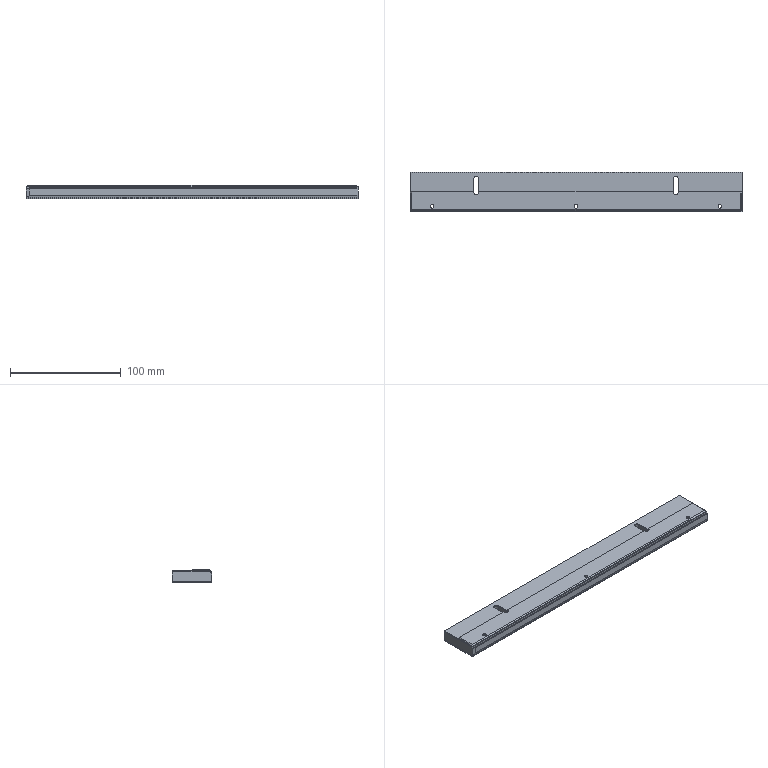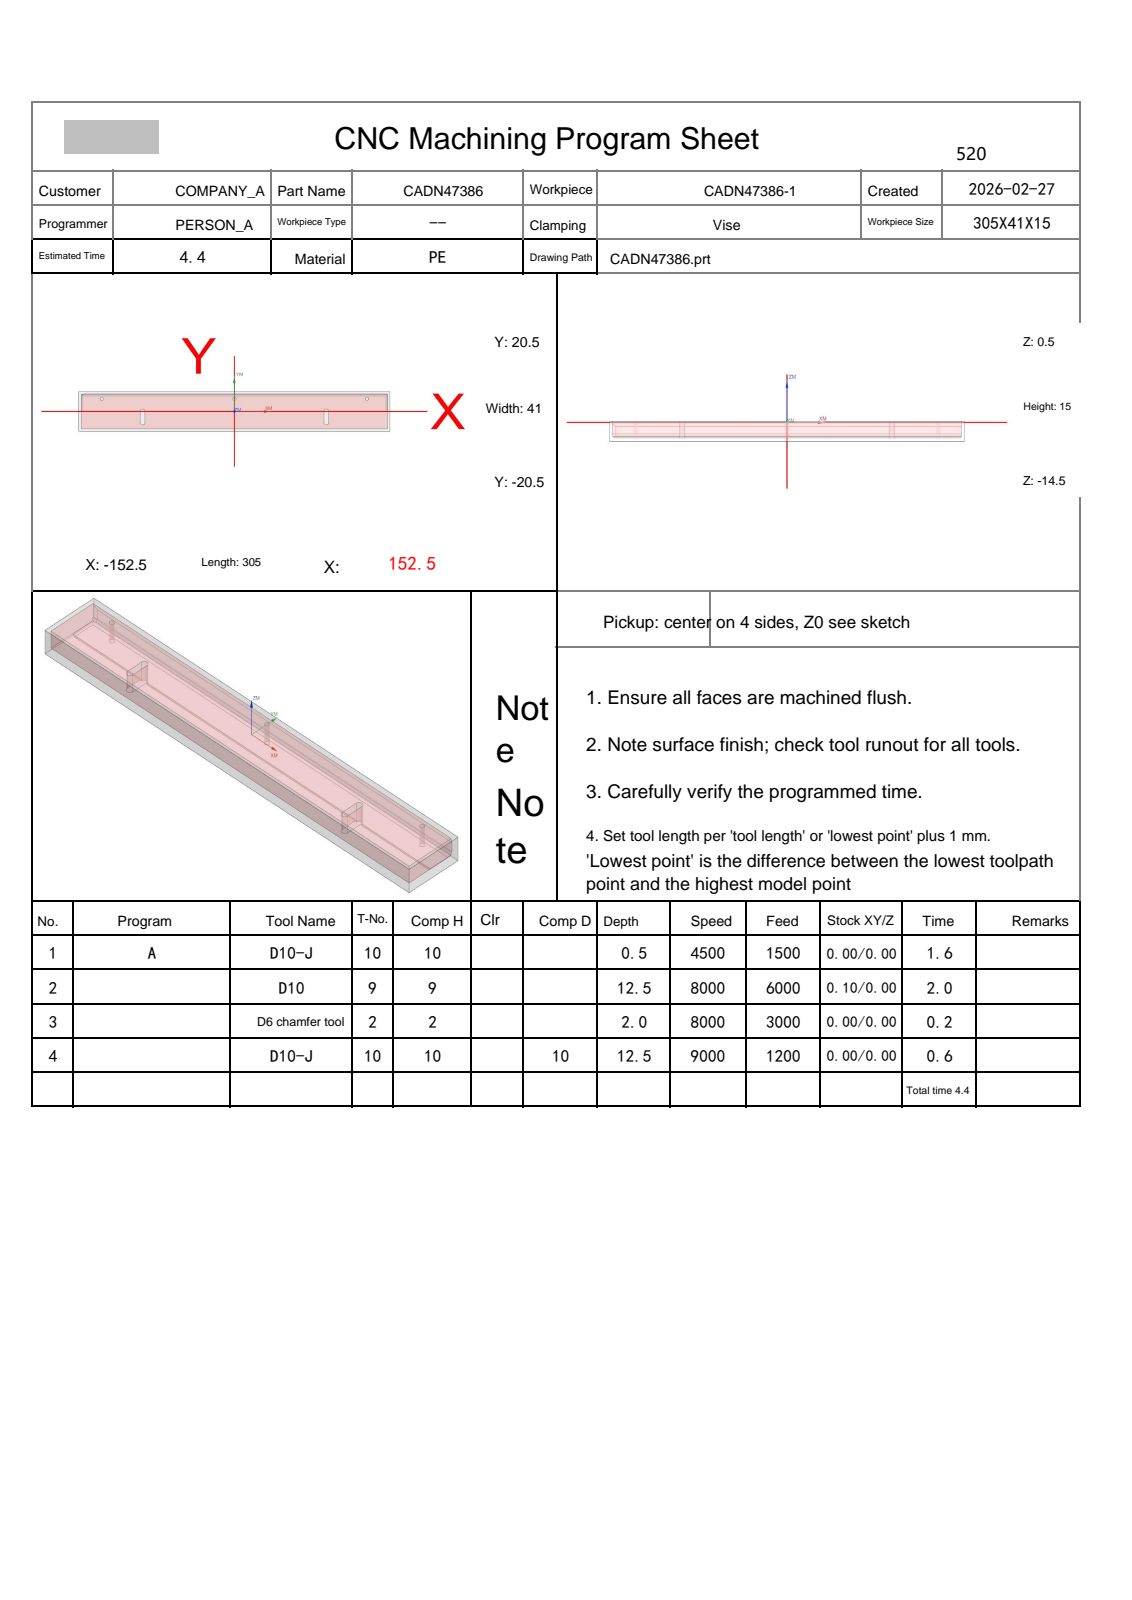NC program | NX | posted by the shop | part box 300 x 36 x 12 mm
Whole program:
%
O0001
(Machine time: 5.25 MIN)
(===Total Tool:3===)
(T10=D10-J  D=10.  R=0.   D-  H10 Z=-12.  )
(T9=D10     D=10.  R=0.   D-  H09 Z=-12.  )
(T2=D6 chamfer tool   D=6.   R=0.   D-  H02 Z=-1.5  )
G80 G90 G17 G49 G40
G91 G28 Z0
M01
N1 T10 M06
(D10-J  D=10. R=0. H=10 ce=0.00 di=0.00)
G00 G90 G54 X140.111 Y28. M03 S4500
G43 H10 Z29.
M08
Z2.
G01 Z0.0 F1500.
X145.111 Y23.
X155. Y13.111
Y3.222
X135.222 Y23.
X125.333
X155. Y-6.667
Y-16.556
X115.444 Y23.
X105.556
X151.556 Y-23.
X141.667
X95.667 Y23.
X85.778
X131.778 Y-23.
X121.889
X75.889 Y23.
X66.
X112. Y-23.
X102.111
X56.111 Y23.
X46.222
X92.222 Y-23.
X82.333
X36.333 Y23.
X26.444
X72.444 Y-23.
X62.556
X16.556 Y23.
X6.667
X52.667 Y-23.
X42.778
X-3.222 Y23.
X-13.111
X32.889 Y-23.
X23.
X-23. Y23.
X-32.889
X13.111 Y-23.
X3.222
X-42.778 Y23.
X-52.667
X-6.667 Y-23.
X-16.556
X-62.556 Y23.
X-72.444
X-26.444 Y-23.
X-36.333
X-82.333 Y23.
X-92.222
X-46.222 Y-23.
X-56.111
X-102.111 Y23.
X-112.
X-66. Y-23.
X-75.889
X-121.889 Y23.
X-131.778
X-85.778 Y-23.
X-95.667
X-141.667 Y23.
X-151.556
X-105.556 Y-23.
X-115.444
X-155. Y16.556
Y6.667
X-125.333 Y-23.
X-135.222
X-155. Y-3.222
Y-13.111
X-145.111 Y-23.
X-140.111 Y-28.
Z2.
G00 Z29.
G91 G28 Z0.0
M05
M09
G91 G28 Z0.0
M01
N2 T09 M06
(D10  D=10. R=0. H=09 ce=0.10 di=0.00)
G00 G90 G54 X-.443 Y23.1 M03 S8000
G43 H09 Z29.
M08
Z.5
G01 X150. Z.333 F6000.
G02 X155.1 Y18. Z.324 I0.0 J-5.1
G01 Y-18. Z.284
G02 X150. Y-23.1 Z.275 I-5.1 J0.0
G01 X-150. Z-.058
G02 X-155.1 Y-18. Z-.067 I0.0 J5.1
G01 Y17.5 Z-.106
G02 X-150.838 Y22.531 Z-.114 I5.1 J0.0
G01 X-147.422 Y23.1 Z-.118
X150. Z-.448
G02 X155.1 Y18. Z-.457 I0.0 J-5.1
G01 Y-18. Z-.497
G02 X150. Y-23.1 Z-.506 I-5.1 J0.0
G01 X-150. Z-.839
G02 X-155.1 Y-18. Z-.848 I0.0 J5.1
G01 Y17.5 Z-.887
G02 X-150.838 Y22.531 Z-.895 I5.1 J0.0
G01 X-147.422 Y23.1 Z-.899
X150. Z-1.23
G02 X155.1 Y18. Z-1.238 I0.0 J-5.1
G01 Y-18. Z-1.278
G02 X150. Y-23.1 Z-1.287 I-5.1 J0.0
G01 X-150. Z-1.62
G02 X-155.1 Y-18. Z-1.629 I0.0 J5.1
G01 Y17.5 Z-1.669
G02 X-150.838 Y22.531 Z-1.677 I5.1 J0.0
G01 X-147.422 Y23.1 Z-1.681
X150. Z-2.011
G02 X155.1 Y18. Z-2.02 I0.0 J-5.1
G01 Y-18. Z-2.06
G02 X150. Y-23.1 Z-2.069 I-5.1 J0.0
G01 X-150. Z-2.402
G02 X-155.1 Y-18. Z-2.411 I0.0 J5.1
G01 Y17.5 Z-2.45
G02 X-150.838 Y22.531 Z-2.458 I5.1 J0.0
G01 X-147.422 Y23.1 Z-2.462
X150. Z-2.792
G02 X155.1 Y18. Z-2.801 I0.0 J-5.1
G01 Y-18. Z-2.841
G02 X150. Y-23.1 Z-2.85 I-5.1 J0.0
G01 X-150. Z-3.183
G02 X-155.1 Y-18. Z-3.192 I0.0 J5.1
G01 Y17.5 Z-3.231
G02 X-150.838 Y22.531 Z-3.239 I5.1 J0.0
G01 X-147.422 Y23.1 Z-3.243
X150. Z-3.573
G02 X155.1 Y18. Z-3.582 I0.0 J-5.1
G01 Y-18. Z-3.622
G02 X150. Y-23.1 Z-3.631 I-5.1 J0.0
G01 X-150. Z-3.964
G02 X-155.1 Y-18. Z-3.973 I0.0 J5.1
G01 Y17.5 Z-4.012
G02 X-150.838 Y22.531 Z-4.02 I5.1 J0.0
G01 X-147.422 Y23.1 Z-4.024
X150. Z-4.355
G02 X155.1 Y18. Z-4.363 I0.0 J-5.1
G01 Y-18. Z-4.403
G02 X150. Y-23.1 Z-4.412 I-5.1 J0.0
G01 X-150. Z-4.745
G02 X-155.1 Y-18. Z-4.754 I0.0 J5.1
G01 Y17.5 Z-4.794
G02 X-150.838 Y22.531 Z-4.802 I5.1 J0.0
G01 X-147.422 Y23.1 Z-4.806
X150. Z-5.136
G02 X155.1 Y18. Z-5.145 I0.0 J-5.1
G01 Y-18. Z-5.185
G02 X150. Y-23.1 Z-5.194 I-5.1 J0.0
G01 X-150. Z-5.527
G02 X-155.1 Y-18. Z-5.536 I0.0 J5.1
G01 Y17.5 Z-5.575
G02 X-150.838 Y22.531 Z-5.583 I5.1 J0.0
G01 X-147.422 Y23.1 Z-5.587
X150. Z-5.917
G02 X155.1 Y18. Z-5.926 I0.0 J-5.1
G01 Y-18. Z-5.966
G02 X150. Y-23.1 Z-5.975 I-5.1 J0.0
G01 X-150. Z-6.308
G02 X-155.1 Y-18. Z-6.317 I0.0 J5.1
G01 Y17.5 Z-6.356
G02 X-150.838 Y22.531 Z-6.364 I5.1 J0.0
G01 X-147.422 Y23.1 Z-6.368
X150. Z-6.698
G02 X155.1 Y18. Z-6.707 I0.0 J-5.1
G01 Y-18. Z-6.747
G02 X150. Y-23.1 Z-6.756 I-5.1 J0.0
G01 X-150. Z-7.089
G02 X-155.1 Y-18. Z-7.098 I0.0 J5.1
G01 Y17.5 Z-7.137
G02 X-150.838 Y22.531 Z-7.145 I5.1 J0.0
G01 X-147.422 Y23.1 Z-7.149
X150. Z-7.48
G02 X155.1 Y18. Z-7.488 I0.0 J-5.1
G01 Y-18. Z-7.528
G02 X150. Y-23.1 Z-7.537 I-5.1 J0.0
G01 X-150. Z-7.87
G02 X-155.1 Y-18. Z-7.879 I0.0 J5.1
G01 Y17.5 Z-7.919
G02 X-150.838 Y22.531 Z-7.927 I5.1 J0.0
G01 X-147.422 Y23.1 Z-7.931
X150. Z-8.261
G02 X155.1 Y18. Z-8.27 I0.0 J-5.1
G01 Y-18. Z-8.31
G02 X150. Y-23.1 Z-8.319 I-5.1 J0.0
G01 X-150. Z-8.652
G02 X-155.1 Y-18. Z-8.661 I0.0 J5.1
G01 Y17.5 Z-8.7
G02 X-150.838 Y22.531 Z-8.708 I5.1 J0.0
G01 X-147.422 Y23.1 Z-8.712
X150. Z-9.042
G02 X155.1 Y18. Z-9.051 I0.0 J-5.1
G01 Y-18. Z-9.091
G02 X150. Y-23.1 Z-9.1 I-5.1 J0.0
G01 X-150. Z-9.433
G02 X-155.1 Y-18. Z-9.442 I0.0 J5.1
G01 Y17.5 Z-9.481
G02 X-150.838 Y22.531 Z-9.489 I5.1 J0.0
G01 X-147.422 Y23.1 Z-9.493
X150. Z-9.823
G02 X155.1 Y18. Z-9.832 I0.0 J-5.1
G01 Y-18. Z-9.872
G02 X150. Y-23.1 Z-9.881 I-5.1 J0.0
G01 X-150. Z-10.214
G02 X-155.1 Y-18. Z-10.223 I0.0 J5.1
G01 Y17.5 Z-10.262
G02 X-150.838 Y22.531 Z-10.27 I5.1 J0.0
G01 X-147.422 Y23.1 Z-10.274
X150. Z-10.605
G02 X155.1 Y18. Z-10.613 I0.0 J-5.1
G01 Y-18. Z-10.653
G02 X150. Y-23.1 Z-10.662 I-5.1 J0.0
G01 X-150. Z-10.995
G02 X-155.1 Y-18. Z-11.004 I0.0 J5.1
G01 Y17.5 Z-11.044
G02 X-150.838 Y22.531 Z-11.052 I5.1 J0.0
G01 X-147.422 Y23.1 Z-11.056
X150. Z-11.386
G02 X155.1 Y18. Z-11.395 I0.0 J-5.1
G01 Y-18. Z-11.435
G02 X150. Y-23.1 Z-11.444 I-5.1 J0.0
G01 X-150. Z-11.777
G02 X-155.1 Y-18. Z-11.786 I0.0 J5.1
G01 Y17.5 Z-11.825
G02 X-150.838 Y22.531 Z-11.833 I5.1 J0.0
G01 X-147.422 Y23.1 Z-11.837
X-.443 Z-12.
X150.
G02 X155.1 Y18. I0.0 J-5.1
G01 Y-18.
G02 X150. Y-23.1 I-5.1 J0.0
G01 X-150.
G02 X-155.1 Y-18. I0.0 J5.1
G01 Y17.5
G02 X-150.838 Y22.531 I5.1 J0.0
G01 X-147.422 Y23.1
X-.443
X.057
Z-11.
G00 Z29.
G91 G28 Z0.0
M05
M09
G91 G28 Z0.0
M01
N3 T02 M06
(D6 chamfer tool  D=6. R=0. H=02 ce=0.00 di=0.00)
G00 G90 G54 X-.25 Y19.378 M03 S8000
G43 H02 Z29.
M08
Z2.099
G01 Z-1.5 F3000.
G03 X-.33 Y19.078 I.52 J-.3
X-.03 Y18.558 I.6 J0.0
G01 X0.0 Y18.55
X150.
G02 X151.3 Y17.25 I0.0 J-1.3
G01 Y-18.
G02 X150. Y-19.3 I-1.3 J0.0
G01 X-150.
G02 X-151.3 Y-18. I0.0 J1.3
G01 Y17.25
G02 X-150. Y18.55 I1.3 J0.0
G01 X0.0
X.03 Y18.558
G03 X.33 Y19.078 I-.3 J.52
X.25 Y19.378 I-.6 J0.0
G01 Z2.099
G00 Z29.
G91 G28 Z0.0
M05
M09
G91 G28 Z0.0
M01
N4 T10 M06
(D10-J  D=10. R=0. H=10 ce=0.00 di=0.00)
G00 G90 G54 X-152.005 Y23.366 M03 S9000
G43 H10 Z29.
M08
Z-11.5
G01 Z-12. F1200.
G41 D10
X-151.956 Y23.172
G03 X-150.986 Y22.418 I.969 J.246
G01 X-150.822 Y22.432
X-147.414 Y23.
X150.
G02 X155. Y18. I0.0 J-5.
G01 Y-18.
G02 X150. Y-23. I-5. J0.0
G01 X-150.
G02 X-155. Y-18. I0.0 J5.
G01 Y17.5
G02 X-150.822 Y22.432 I5. J0.0
G01 X-150.329 Y22.514
G03 X-149.493 Y23.501 I-.164 J.986
G01 X-149.507 Y23.665
G40 X-149.54 Y23.862
Z-11.5
G00 Z29.
M05
M09
G91 G28 Z0.0
G91 G28 Y0.0
M30
%